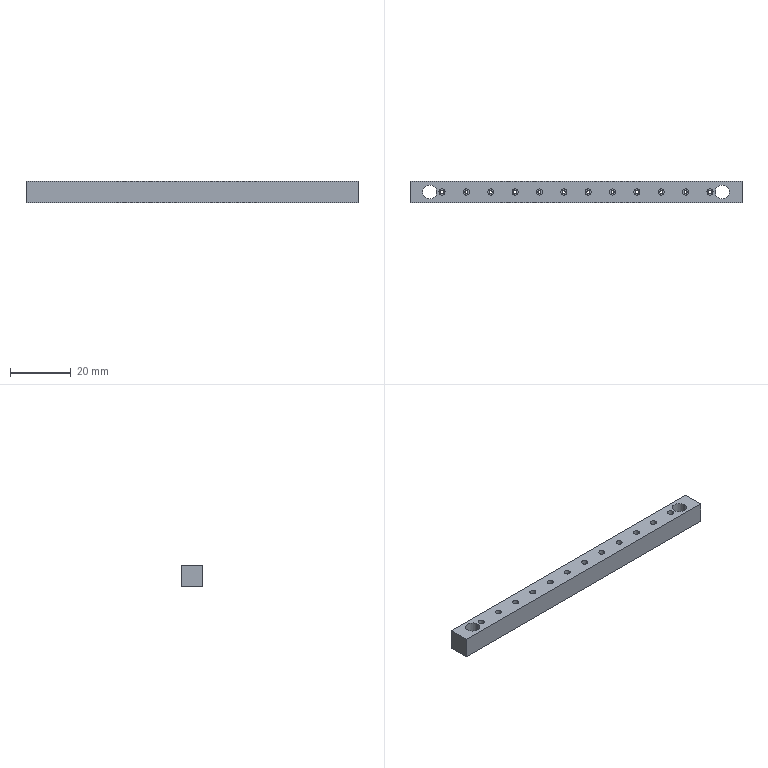Part | SolidWorks | features BaseBody 1 | 1 solid | 70 faces | box 109 x 7 x 7 mm | volume 4929 mm3 | cylinder 52 | plane 18 | commonest cylinder face diameters 1 x24 2 x24 4.6 x4